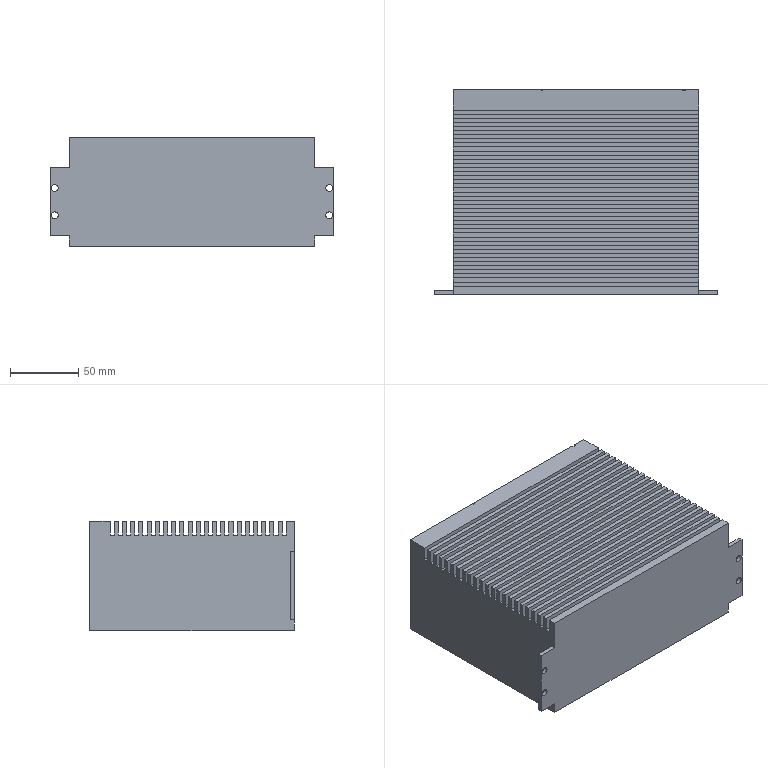Part | SolidWorks | features ICE 6, Extrusion 1 | 1 solid | 151 faces | box 208 x 150 x 80 mm | volume 2042108 mm3 | plane 131 | cylinder 20 | commonest cylinder face diameters 4 x12 5 x8